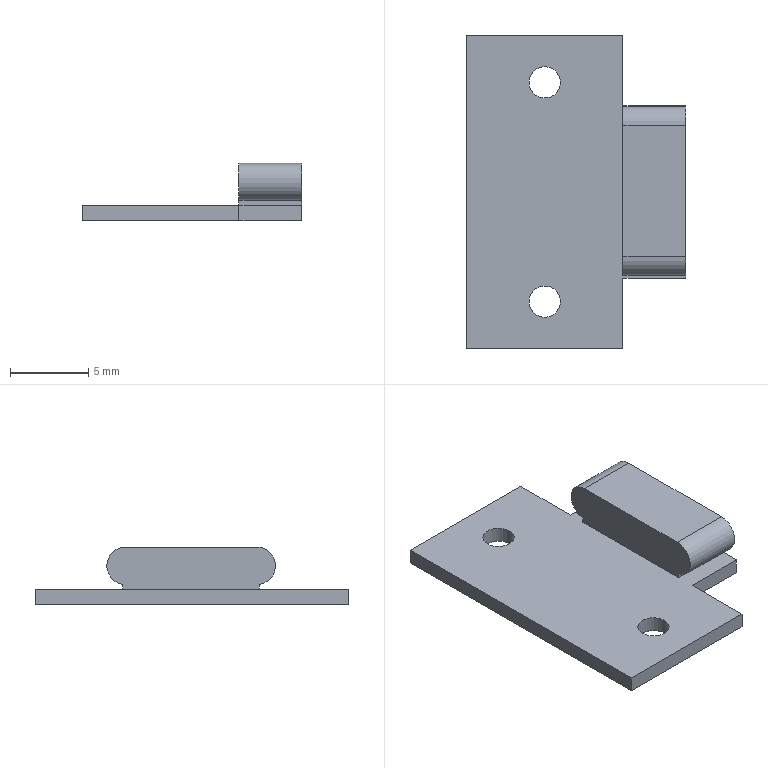Part | SolidWorks | features ICE 4, Extrusion 1 | 1 solid | 25 faces | box 14 x 20 x 3.696 mm | volume 327.493 mm3 | plane 19 | cylinder 6 | commonest cylinder face diameters 2 x4 2.393 x2
STEP:
#1=CARTESIAN_POINT('',(-1.,-7.,1.));
#2=VERTEX_POINT('',#1);
#3=CARTESIAN_POINT('',(1.,-7.,1.));
#4=VERTEX_POINT('',#3);
#5=CARTESIAN_POINT('',(0.,-7.,1.));
#6=DIRECTION('',(0.,0.,1.));
#7=DIRECTION('',(1.,0.,0.));
#8=AXIS2_PLACEMENT_3D('',#5,#6,#7);
#9=CIRCLE('',#8,1.);
#10=EDGE_CURVE('',#2,#4,#9,.T.);
#11=ORIENTED_EDGE('',*,*,#10,.T.);
#12=CARTESIAN_POINT('',(1.,-7.,0.));
#13=VERTEX_POINT('',#12);
#14=CARTESIAN_POINT('',(1.,-7.,1.));
#15=DIRECTION('',(0.,0.,-1.));
#16=VECTOR('',#15,1000.);
#17=LINE('',#14,#16);
#18=EDGE_CURVE('',#4,#13,#17,.T.);
#19=ORIENTED_EDGE('',*,*,#18,.T.);
#20=CARTESIAN_POINT('',(-1.,-7.,0.));
#21=VERTEX_POINT('',#20);
#22=CARTESIAN_POINT('',(0.,-7.,0.));
#23=DIRECTION('',(0.,0.,1.));
#24=DIRECTION('',(1.,0.,0.));
#25=AXIS2_PLACEMENT_3D('',#22,#23,#24);
#26=CIRCLE('',#25,1.);
#27=EDGE_CURVE('',#21,#13,#26,.T.);
#28=ORIENTED_EDGE('',*,*,#27,.F.);
#29=CARTESIAN_POINT('',(-1.,-7.,1.));
#30=DIRECTION('',(0.,0.,-1.));
#31=VECTOR('',#30,1000.);
#32=LINE('',#29,#31);
#33=EDGE_CURVE('',#2,#21,#32,.T.);
#34=ORIENTED_EDGE('',*,*,#33,.F.);
#35=EDGE_LOOP('',(#11,#19,#28,#34));
#36=FACE_OUTER_BOUND('',#35,.T.);
#37=CARTESIAN_POINT('',(0.,-7.,1.));
#38=DIRECTION('',(0.,0.,-1.));
#39=DIRECTION('',(-1.,0.,0.));
#40=AXIS2_PLACEMENT_3D('',#37,#38,#39);
#41=CYLINDRICAL_SURFACE('',#40,1.);
#42=ADVANCED_FACE('',(#36),#41,.F.);
#43=CARTESIAN_POINT('',(-1.,7.,1.));
#44=VERTEX_POINT('',#43);
#45=CARTESIAN_POINT('',(1.,7.,1.));
#46=VERTEX_POINT('',#45);
#47=CARTESIAN_POINT('',(0.,7.,1.));
#48=DIRECTION('',(0.,0.,1.));
#49=DIRECTION('',(1.,0.,0.));
#50=AXIS2_PLACEMENT_3D('',#47,#48,#49);
#51=CIRCLE('',#50,1.);
#52=EDGE_CURVE('',#44,#46,#51,.T.);
#53=ORIENTED_EDGE('',*,*,#52,.T.);
#54=CARTESIAN_POINT('',(1.,7.,0.));
#55=VERTEX_POINT('',#54);
#56=CARTESIAN_POINT('',(1.,7.,1.));
#57=DIRECTION('',(0.,0.,-1.));
#58=VECTOR('',#57,1000.);
#59=LINE('',#56,#58);
#60=EDGE_CURVE('',#46,#55,#59,.T.);
#61=ORIENTED_EDGE('',*,*,#60,.T.);
#62=CARTESIAN_POINT('',(-1.,7.,0.));
#63=VERTEX_POINT('',#62);
#64=CARTESIAN_POINT('',(0.,7.,0.));
#65=DIRECTION('',(0.,0.,1.));
#66=DIRECTION('',(1.,0.,0.));
#67=AXIS2_PLACEMENT_3D('',#64,#65,#66);
#68=CIRCLE('',#67,1.);
#69=EDGE_CURVE('',#63,#55,#68,.T.);
#70=ORIENTED_EDGE('',*,*,#69,.F.);
#71=CARTESIAN_POINT('',(-1.,7.,1.));
#72=DIRECTION('',(0.,0.,-1.));
#73=VECTOR('',#72,1000.);
#74=LINE('',#71,#73);
#75=EDGE_CURVE('',#44,#63,#74,.T.);
#76=ORIENTED_EDGE('',*,*,#75,.F.);
#77=EDGE_LOOP('',(#53,#61,#70,#76));
#78=FACE_OUTER_BOUND('',#77,.T.);
#79=CARTESIAN_POINT('',(0.,7.,1.));
#80=DIRECTION('',(0.,0.,-1.));
#81=DIRECTION('',(-1.,0.,0.));
#82=AXIS2_PLACEMENT_3D('',#79,#80,#81);
#83=CYLINDRICAL_SURFACE('',#82,1.);
#84=ADVANCED_FACE('',(#78),#83,.F.);
#85=CARTESIAN_POINT('',(5.,-4.302,1.));
#86=VERTEX_POINT('',#85);
#87=CARTESIAN_POINT('',(9.,-4.302,1.));
#88=VERTEX_POINT('',#87);
#89=CARTESIAN_POINT('',(5.,-4.302,1.));
#90=DIRECTION('',(1.,0.,0.));
#91=VECTOR('',#90,1000.);
#92=LINE('',#89,#91);
#93=EDGE_CURVE('',#86,#88,#92,.T.);
#94=ORIENTED_EDGE('',*,*,#93,.F.);
#95=CARTESIAN_POINT('',(5.,4.41,1.));
#96=VERTEX_POINT('',#95);
#97=CARTESIAN_POINT('',(5.,-4.302,1.));
#98=DIRECTION('',(0.,1.,0.));
#99=VECTOR('',#98,1000.);
#100=LINE('',#97,#99);
#101=EDGE_CURVE('',#86,#96,#100,.T.);
#102=ORIENTED_EDGE('',*,*,#101,.T.);
#103=CARTESIAN_POINT('',(9.,4.41,1.));
#104=VERTEX_POINT('',#103);
#105=CARTESIAN_POINT('',(5.,4.41,1.));
#106=DIRECTION('',(1.,0.,0.));
#107=VECTOR('',#106,1000.);
#108=LINE('',#105,#107);
#109=EDGE_CURVE('',#96,#104,#108,.T.);
#110=ORIENTED_EDGE('',*,*,#109,.T.);
#111=CARTESIAN_POINT('',(9.,5.5,1.));
#112=VERTEX_POINT('',#111);
#113=CARTESIAN_POINT('',(9.,-5.5,1.));
#114=DIRECTION('',(0.,1.,0.));
#115=VECTOR('',#114,1000.);
#116=LINE('',#113,#115);
#117=EDGE_CURVE('',#104,#112,#116,.T.);
#118=ORIENTED_EDGE('',*,*,#117,.T.);
#119=CARTESIAN_POINT('',(5.,5.5,1.));
#120=VERTEX_POINT('',#119);
#121=CARTESIAN_POINT('',(-1.,5.5,1.));
#122=DIRECTION('',(1.,0.,0.));
#123=VECTOR('',#122,1000.);
#124=LINE('',#121,#123);
#125=EDGE_CURVE('',#120,#112,#124,.T.);
#126=ORIENTED_EDGE('',*,*,#125,.F.);
#127=CARTESIAN_POINT('',(5.,10.,1.));
#128=VERTEX_POINT('',#127);
#129=CARTESIAN_POINT('',(5.,10.,1.));
#130=DIRECTION('',(0.,1.,0.));
#131=VECTOR('',#130,1000.);
#132=LINE('',#129,#131);
#133=EDGE_CURVE('',#120,#128,#132,.T.);
#134=ORIENTED_EDGE('',*,*,#133,.T.);
#135=CARTESIAN_POINT('',(-5.,10.,1.));
#136=VERTEX_POINT('',#135);
#137=CARTESIAN_POINT('',(-5.,10.,1.));
#138=DIRECTION('',(-1.,0.,0.));
#139=VECTOR('',#138,1000.);
#140=LINE('',#137,#139);
#141=EDGE_CURVE('',#128,#136,#140,.T.);
#142=ORIENTED_EDGE('',*,*,#141,.T.);
#143=CARTESIAN_POINT('',(-5.,-10.,1.));
#144=VERTEX_POINT('',#143);
#145=CARTESIAN_POINT('',(-5.,10.,1.));
#146=DIRECTION('',(0.,-1.,0.));
#147=VECTOR('',#146,1000.);
#148=LINE('',#145,#147);
#149=EDGE_CURVE('',#136,#144,#148,.T.);
#150=ORIENTED_EDGE('',*,*,#149,.T.);
#151=CARTESIAN_POINT('',(5.,-10.,1.));
#152=VERTEX_POINT('',#151);
#153=CARTESIAN_POINT('',(-5.,-10.,1.));
#154=DIRECTION('',(1.,0.,0.));
#155=VECTOR('',#154,1000.);
#156=LINE('',#153,#155);
#157=EDGE_CURVE('',#144,#152,#156,.T.);
#158=ORIENTED_EDGE('',*,*,#157,.T.);
#159=CARTESIAN_POINT('',(5.,-5.5,1.));
#160=VERTEX_POINT('',#159);
#161=CARTESIAN_POINT('',(5.,-5.5,1.));
#162=DIRECTION('',(0.,1.,0.));
#163=VECTOR('',#162,1000.);
#164=LINE('',#161,#163);
#165=EDGE_CURVE('',#152,#160,#164,.T.);
#166=ORIENTED_EDGE('',*,*,#165,.T.);
#167=CARTESIAN_POINT('',(9.,-5.5,1.));
#168=VERTEX_POINT('',#167);
#169=CARTESIAN_POINT('',(-1.,-5.5,1.));
#170=DIRECTION('',(1.,0.,0.));
#171=VECTOR('',#170,1000.);
#172=LINE('',#169,#171);
#173=EDGE_CURVE('',#160,#168,#172,.T.);
#174=ORIENTED_EDGE('',*,*,#173,.T.);
#175=CARTESIAN_POINT('',(9.,-5.5,1.));
#176=DIRECTION('',(0.,1.,0.));
#177=VECTOR('',#176,1000.);
#178=LINE('',#175,#177);
#179=EDGE_CURVE('',#168,#88,#178,.T.);
#180=ORIENTED_EDGE('',*,*,#179,.T.);
#181=EDGE_LOOP('',(#94,#102,#110,#118,#126,#134,#142,#150,#158,#166,#174,#180));
#182=FACE_OUTER_BOUND('',#181,.T.);
#183=ORIENTED_EDGE('',*,*,#52,.F.);
#184=CARTESIAN_POINT('',(0.,7.,1.));
#185=DIRECTION('',(0.,0.,1.));
#186=DIRECTION('',(1.,0.,0.));
#187=AXIS2_PLACEMENT_3D('',#184,#185,#186);
#188=CIRCLE('',#187,1.);
#189=EDGE_CURVE('',#46,#44,#188,.T.);
#190=ORIENTED_EDGE('',*,*,#189,.F.);
#191=EDGE_LOOP('',(#183,#190));
#192=FACE_BOUND('',#191,.T.);
#193=ORIENTED_EDGE('',*,*,#10,.F.);
#194=CARTESIAN_POINT('',(0.,-7.,1.));
#195=DIRECTION('',(0.,0.,1.));
#196=DIRECTION('',(1.,0.,0.));
#197=AXIS2_PLACEMENT_3D('',#194,#195,#196);
#198=CIRCLE('',#197,1.);
#199=EDGE_CURVE('',#4,#2,#198,.T.);
#200=ORIENTED_EDGE('',*,*,#199,.F.);
#201=EDGE_LOOP('',(#193,#200));
#202=FACE_BOUND('',#201,.T.);
#203=CARTESIAN_POINT('',(0.,0.,1.));
#204=DIRECTION('',(0.,0.,1.));
#205=DIRECTION('',(1.,0.,0.));
#206=AXIS2_PLACEMENT_3D('',#203,#204,#205);
#207=PLANE('',#206);
#208=ADVANCED_FACE('',(#182,#192,#202),#207,.T.);
#209=CARTESIAN_POINT('',(5.,-10.,0.));
#210=VERTEX_POINT('',#209);
#211=CARTESIAN_POINT('',(5.,-5.5,0.));
#212=VERTEX_POINT('',#211);
#213=CARTESIAN_POINT('',(5.,-5.5,0.));
#214=DIRECTION('',(0.,1.,0.));
#215=VECTOR('',#214,1000.);
#216=LINE('',#213,#215);
#217=EDGE_CURVE('',#210,#212,#216,.T.);
#218=ORIENTED_EDGE('',*,*,#217,.F.);
#219=CARTESIAN_POINT('',(-5.,-10.,0.));
#220=VERTEX_POINT('',#219);
#221=CARTESIAN_POINT('',(-5.,-10.,0.));
#222=DIRECTION('',(1.,0.,0.));
#223=VECTOR('',#222,1000.);
#224=LINE('',#221,#223);
#225=EDGE_CURVE('',#220,#210,#224,.T.);
#226=ORIENTED_EDGE('',*,*,#225,.F.);
#227=CARTESIAN_POINT('',(-5.,10.,0.));
#228=VERTEX_POINT('',#227);
#229=CARTESIAN_POINT('',(-5.,10.,0.));
#230=DIRECTION('',(0.,-1.,0.));
#231=VECTOR('',#230,1000.);
#232=LINE('',#229,#231);
#233=EDGE_CURVE('',#228,#220,#232,.T.);
#234=ORIENTED_EDGE('',*,*,#233,.F.);
#235=CARTESIAN_POINT('',(5.,10.,0.));
#236=VERTEX_POINT('',#235);
#237=CARTESIAN_POINT('',(-5.,10.,0.));
#238=DIRECTION('',(-1.,0.,0.));
#239=VECTOR('',#238,1000.);
#240=LINE('',#237,#239);
#241=EDGE_CURVE('',#236,#228,#240,.T.);
#242=ORIENTED_EDGE('',*,*,#241,.F.);
#243=CARTESIAN_POINT('',(5.,5.5,0.));
#244=VERTEX_POINT('',#243);
#245=CARTESIAN_POINT('',(5.,10.,0.));
#246=DIRECTION('',(0.,1.,0.));
#247=VECTOR('',#246,1000.);
#248=LINE('',#245,#247);
#249=EDGE_CURVE('',#244,#236,#248,.T.);
#250=ORIENTED_EDGE('',*,*,#249,.F.);
#251=CARTESIAN_POINT('',(9.,5.5,0.));
#252=VERTEX_POINT('',#251);
#253=CARTESIAN_POINT('',(5.,5.5,0.));
#254=DIRECTION('',(-1.,0.,0.));
#255=VECTOR('',#254,1000.);
#256=LINE('',#253,#255);
#257=EDGE_CURVE('',#252,#244,#256,.T.);
#258=ORIENTED_EDGE('',*,*,#257,.F.);
#259=CARTESIAN_POINT('',(9.,-5.5,0.));
#260=VERTEX_POINT('',#259);
#261=CARTESIAN_POINT('',(9.,5.5,0.));
#262=DIRECTION('',(0.,1.,0.));
#263=VECTOR('',#262,1000.);
#264=LINE('',#261,#263);
#265=EDGE_CURVE('',#260,#252,#264,.T.);
#266=ORIENTED_EDGE('',*,*,#265,.F.);
#267=CARTESIAN_POINT('',(5.,-5.5,0.));
#268=DIRECTION('',(1.,0.,0.));
#269=VECTOR('',#268,1000.);
#270=LINE('',#267,#269);
#271=EDGE_CURVE('',#212,#260,#270,.T.);
#272=ORIENTED_EDGE('',*,*,#271,.F.);
#273=EDGE_LOOP('',(#218,#226,#234,#242,#250,#258,#266,#272));
#274=FACE_OUTER_BOUND('',#273,.T.);
#275=ORIENTED_EDGE('',*,*,#69,.T.);
#276=CARTESIAN_POINT('',(0.,7.,0.));
#277=DIRECTION('',(0.,0.,1.));
#278=DIRECTION('',(1.,0.,0.));
#279=AXIS2_PLACEMENT_3D('',#276,#277,#278);
#280=CIRCLE('',#279,1.);
#281=EDGE_CURVE('',#55,#63,#280,.T.);
#282=ORIENTED_EDGE('',*,*,#281,.T.);
#283=EDGE_LOOP('',(#275,#282));
#284=FACE_BOUND('',#283,.T.);
#285=ORIENTED_EDGE('',*,*,#27,.T.);
#286=CARTESIAN_POINT('',(0.,-7.,0.));
#287=DIRECTION('',(0.,0.,1.));
#288=DIRECTION('',(1.,0.,0.));
#289=AXIS2_PLACEMENT_3D('',#286,#287,#288);
#290=CIRCLE('',#289,1.);
#291=EDGE_CURVE('',#13,#21,#290,.T.);
#292=ORIENTED_EDGE('',*,*,#291,.T.);
#293=EDGE_LOOP('',(#285,#292));
#294=FACE_BOUND('',#293,.T.);
#295=CARTESIAN_POINT('',(0.,0.,0.));
#296=DIRECTION('',(0.,0.,1.));
#297=DIRECTION('',(1.,0.,0.));
#298=AXIS2_PLACEMENT_3D('',#295,#296,#297);
#299=PLANE('',#298);
#300=ADVANCED_FACE('',(#274,#284,#294),#299,.F.);
#301=ORIENTED_EDGE('',*,*,#217,.T.);
#302=CARTESIAN_POINT('',(5.,-5.5,1.));
#303=DIRECTION('',(0.,0.,-1.));
#304=VECTOR('',#303,1000.);
#305=LINE('',#302,#304);
#306=EDGE_CURVE('',#160,#212,#305,.T.);
#307=ORIENTED_EDGE('',*,*,#306,.F.);
#308=ORIENTED_EDGE('',*,*,#165,.F.);
#309=CARTESIAN_POINT('',(5.,-10.,1.));
#310=DIRECTION('',(0.,0.,-1.));
#311=VECTOR('',#310,1000.);
#312=LINE('',#309,#311);
#313=EDGE_CURVE('',#152,#210,#312,.T.);
#314=ORIENTED_EDGE('',*,*,#313,.T.);
#315=EDGE_LOOP('',(#301,#307,#308,#314));
#316=FACE_OUTER_BOUND('',#315,.T.);
#317=CARTESIAN_POINT('',(5.,-5.5,1.));
#318=DIRECTION('',(-1.,0.,0.));
#319=DIRECTION('',(0.,-1.,0.));
#320=AXIS2_PLACEMENT_3D('',#317,#318,#319);
#321=PLANE('',#320);
#322=ADVANCED_FACE('',(#316),#321,.F.);
#323=CARTESIAN_POINT('',(9.,-5.5,1.));
#324=DIRECTION('',(0.,0.,-1.));
#325=VECTOR('',#324,1000.);
#326=LINE('',#323,#325);
#327=EDGE_CURVE('',#168,#260,#326,.T.);
#328=ORIENTED_EDGE('',*,*,#327,.F.);
#329=ORIENTED_EDGE('',*,*,#173,.F.);
#330=ORIENTED_EDGE('',*,*,#306,.T.);
#331=ORIENTED_EDGE('',*,*,#271,.T.);
#332=EDGE_LOOP('',(#328,#329,#330,#331));
#333=FACE_OUTER_BOUND('',#332,.T.);
#334=CARTESIAN_POINT('',(5.,-5.5,1.));
#335=DIRECTION('',(0.,1.,0.));
#336=DIRECTION('',(-1.,0.,0.));
#337=AXIS2_PLACEMENT_3D('',#334,#335,#336);
#338=PLANE('',#337);
#339=ADVANCED_FACE('',(#333),#338,.F.);
#340=CARTESIAN_POINT('',(9.,-4.14,3.696));
#341=VERTEX_POINT('',#340);
#342=CARTESIAN_POINT('',(9.,-4.302,1.315));
#343=VERTEX_POINT('',#342);
#344=CARTESIAN_POINT('',(9.,-4.14,2.5));
#345=DIRECTION('',(1.,0.,0.));
#346=DIRECTION('',(0.,0.,-1.));
#347=AXIS2_PLACEMENT_3D('',#344,#345,#346);
#348=CIRCLE('',#347,1.196);
#349=EDGE_CURVE('',#341,#343,#348,.T.);
#350=ORIENTED_EDGE('',*,*,#349,.T.);
#351=CARTESIAN_POINT('',(9.,-4.302,1.607));
#352=DIRECTION('',(0.,0.,-1.));
#353=VECTOR('',#352,1000.);
#354=LINE('',#351,#353);
#355=EDGE_CURVE('',#343,#88,#354,.T.);
#356=ORIENTED_EDGE('',*,*,#355,.T.);
#357=ORIENTED_EDGE('',*,*,#179,.F.);
#358=ORIENTED_EDGE('',*,*,#327,.T.);
#359=ORIENTED_EDGE('',*,*,#265,.T.);
#360=CARTESIAN_POINT('',(9.,5.5,1.));
#361=DIRECTION('',(0.,0.,-1.));
#362=VECTOR('',#361,1000.);
#363=LINE('',#360,#362);
#364=EDGE_CURVE('',#112,#252,#363,.T.);
#365=ORIENTED_EDGE('',*,*,#364,.F.);
#366=ORIENTED_EDGE('',*,*,#117,.F.);
#367=CARTESIAN_POINT('',(9.,4.41,1.315));
#368=VERTEX_POINT('',#367);
#369=CARTESIAN_POINT('',(9.,4.41,1.607));
#370=DIRECTION('',(0.,0.,1.));
#371=VECTOR('',#370,1000.);
#372=LINE('',#369,#371);
#373=EDGE_CURVE('',#104,#368,#372,.T.);
#374=ORIENTED_EDGE('',*,*,#373,.T.);
#375=CARTESIAN_POINT('',(9.,4.248,3.696));
#376=VERTEX_POINT('',#375);
#377=CARTESIAN_POINT('',(9.,4.248,2.5));
#378=DIRECTION('',(1.,0.,0.));
#379=DIRECTION('',(0.,0.,-1.));
#380=AXIS2_PLACEMENT_3D('',#377,#378,#379);
#381=CIRCLE('',#380,1.196);
#382=EDGE_CURVE('',#368,#376,#381,.T.);
#383=ORIENTED_EDGE('',*,*,#382,.T.);
#384=CARTESIAN_POINT('',(9.,4.248,3.696));
#385=DIRECTION('',(0.,-1.,0.));
#386=VECTOR('',#385,1000.);
#387=LINE('',#384,#386);
#388=EDGE_CURVE('',#376,#341,#387,.T.);
#389=ORIENTED_EDGE('',*,*,#388,.T.);
#390=EDGE_LOOP('',(#350,#356,#357,#358,#359,#365,#366,#374,#383,#389));
#391=FACE_OUTER_BOUND('',#390,.T.);
#392=CARTESIAN_POINT('',(9.,4.573,2.105));
#393=VERTEX_POINT('',#392);
#394=CARTESIAN_POINT('',(9.,4.573,2.809));
#395=VERTEX_POINT('',#394);
#396=CARTESIAN_POINT('',(9.,4.573,2.809));
#397=DIRECTION('',(0.,0.,1.));
#398=VECTOR('',#397,1000.);
#399=LINE('',#396,#398);
#400=EDGE_CURVE('',#393,#395,#399,.T.);
#401=ORIENTED_EDGE('',*,*,#400,.F.);
#402=CARTESIAN_POINT('',(9.,-4.464,2.105));
#403=VERTEX_POINT('',#402);
#404=CARTESIAN_POINT('',(9.,4.573,2.105));
#405=DIRECTION('',(0.,1.,0.));
#406=VECTOR('',#405,1000.);
#407=LINE('',#404,#406);
#408=EDGE_CURVE('',#403,#393,#407,.T.);
#409=ORIENTED_EDGE('',*,*,#408,.F.);
#410=CARTESIAN_POINT('',(9.,-4.464,2.809));
#411=VERTEX_POINT('',#410);
#412=CARTESIAN_POINT('',(9.,-4.464,2.809));
#413=DIRECTION('',(0.,0.,-1.));
#414=VECTOR('',#413,1000.);
#415=LINE('',#412,#414);
#416=EDGE_CURVE('',#411,#403,#415,.T.);
#417=ORIENTED_EDGE('',*,*,#416,.F.);
#418=CARTESIAN_POINT('',(9.,4.573,2.809));
#419=DIRECTION('',(0.,-1.,0.));
#420=VECTOR('',#419,1000.);
#421=LINE('',#418,#420);
#422=EDGE_CURVE('',#395,#411,#421,.T.);
#423=ORIENTED_EDGE('',*,*,#422,.F.);
#424=EDGE_LOOP('',(#401,#409,#417,#423));
#425=FACE_BOUND('',#424,.T.);
#426=CARTESIAN_POINT('',(9.,5.5,1.));
#427=DIRECTION('',(-1.,0.,0.));
#428=DIRECTION('',(0.,0.,1.));
#429=AXIS2_PLACEMENT_3D('',#426,#427,#428);
#430=PLANE('',#429);
#431=ADVANCED_FACE('',(#391,#425),#430,.F.);
#432=CARTESIAN_POINT('',(5.,5.5,1.));
#433=DIRECTION('',(0.,0.,-1.));
#434=VECTOR('',#433,1000.);
#435=LINE('',#432,#434);
#436=EDGE_CURVE('',#120,#244,#435,.T.);
#437=ORIENTED_EDGE('',*,*,#436,.F.);
#438=ORIENTED_EDGE('',*,*,#125,.T.);
#439=ORIENTED_EDGE('',*,*,#364,.T.);
#440=ORIENTED_EDGE('',*,*,#257,.T.);
#441=EDGE_LOOP('',(#437,#438,#439,#440));
#442=FACE_OUTER_BOUND('',#441,.T.);
#443=CARTESIAN_POINT('',(5.,5.5,1.));
#444=DIRECTION('',(0.,-1.,0.));
#445=DIRECTION('',(0.,0.,-1.));
#446=AXIS2_PLACEMENT_3D('',#443,#444,#445);
#447=PLANE('',#446);
#448=ADVANCED_FACE('',(#442),#447,.F.);
#449=ORIENTED_EDGE('',*,*,#249,.T.);
#450=CARTESIAN_POINT('',(5.,10.,1.));
#451=DIRECTION('',(0.,0.,-1.));
#452=VECTOR('',#451,1000.);
#453=LINE('',#450,#452);
#454=EDGE_CURVE('',#128,#236,#453,.T.);
#455=ORIENTED_EDGE('',*,*,#454,.F.);
#456=ORIENTED_EDGE('',*,*,#133,.F.);
#457=ORIENTED_EDGE('',*,*,#436,.T.);
#458=EDGE_LOOP('',(#449,#455,#456,#457));
#459=FACE_OUTER_BOUND('',#458,.T.);
#460=CARTESIAN_POINT('',(5.,10.,1.));
#461=DIRECTION('',(-1.,0.,0.));
#462=DIRECTION('',(0.,-1.,0.));
#463=AXIS2_PLACEMENT_3D('',#460,#461,#462);
#464=PLANE('',#463);
#465=ADVANCED_FACE('',(#459),#464,.F.);
#466=ORIENTED_EDGE('',*,*,#241,.T.);
#467=CARTESIAN_POINT('',(-5.,10.,1.));
#468=DIRECTION('',(0.,0.,-1.));
#469=VECTOR('',#468,1000.);
#470=LINE('',#467,#469);
#471=EDGE_CURVE('',#136,#228,#470,.T.);
#472=ORIENTED_EDGE('',*,*,#471,.F.);
#473=ORIENTED_EDGE('',*,*,#141,.F.);
#474=ORIENTED_EDGE('',*,*,#454,.T.);
#475=EDGE_LOOP('',(#466,#472,#473,#474));
#476=FACE_OUTER_BOUND('',#475,.T.);
#477=CARTESIAN_POINT('',(-5.,10.,1.));
#478=DIRECTION('',(0.,-1.,0.));
#479=DIRECTION('',(0.,0.,-1.));
#480=AXIS2_PLACEMENT_3D('',#477,#478,#479);
#481=PLANE('',#480);
#482=ADVANCED_FACE('',(#476),#481,.F.);
#483=ORIENTED_EDGE('',*,*,#233,.T.);
#484=CARTESIAN_POINT('',(-5.,-10.,1.));
#485=DIRECTION('',(0.,0.,-1.));
#486=VECTOR('',#485,1000.);
#487=LINE('',#484,#486);
#488=EDGE_CURVE('',#144,#220,#487,.T.);
#489=ORIENTED_EDGE('',*,*,#488,.F.);
#490=ORIENTED_EDGE('',*,*,#149,.F.);
#491=ORIENTED_EDGE('',*,*,#471,.T.);
#492=EDGE_LOOP('',(#483,#489,#490,#491));
#493=FACE_OUTER_BOUND('',#492,.T.);
#494=CARTESIAN_POINT('',(-5.,10.,1.));
#495=DIRECTION('',(1.,0.,0.));
#496=DIRECTION('',(0.,1.,0.));
#497=AXIS2_PLACEMENT_3D('',#494,#495,#496);
#498=PLANE('',#497);
#499=ADVANCED_FACE('',(#493),#498,.F.);
#500=ORIENTED_EDGE('',*,*,#225,.T.);
#501=ORIENTED_EDGE('',*,*,#313,.F.);
#502=ORIENTED_EDGE('',*,*,#157,.F.);
#503=ORIENTED_EDGE('',*,*,#488,.T.);
#504=EDGE_LOOP('',(#500,#501,#502,#503));
#505=FACE_OUTER_BOUND('',#504,.T.);
#506=CARTESIAN_POINT('',(-5.,-10.,1.));
#507=DIRECTION('',(0.,1.,0.));
#508=DIRECTION('',(0.,0.,1.));
#509=AXIS2_PLACEMENT_3D('',#506,#507,#508);
#510=PLANE('',#509);
#511=ADVANCED_FACE('',(#505),#510,.F.);
#512=ORIENTED_EDGE('',*,*,#60,.F.);
#513=ORIENTED_EDGE('',*,*,#189,.T.);
#514=ORIENTED_EDGE('',*,*,#75,.T.);
#515=ORIENTED_EDGE('',*,*,#281,.F.);
#516=EDGE_LOOP('',(#512,#513,#514,#515));
#517=FACE_OUTER_BOUND('',#516,.T.);
#518=CARTESIAN_POINT('',(0.,7.,1.));
#519=DIRECTION('',(0.,0.,-1.));
#520=DIRECTION('',(-1.,0.,0.));
#521=AXIS2_PLACEMENT_3D('',#518,#519,#520);
#522=CYLINDRICAL_SURFACE('',#521,1.);
#523=ADVANCED_FACE('',(#517),#522,.F.);
#524=ORIENTED_EDGE('',*,*,#18,.F.);
#525=ORIENTED_EDGE('',*,*,#199,.T.);
#526=ORIENTED_EDGE('',*,*,#33,.T.);
#527=ORIENTED_EDGE('',*,*,#291,.F.);
#528=EDGE_LOOP('',(#524,#525,#526,#527));
#529=FACE_OUTER_BOUND('',#528,.T.);
#530=CARTESIAN_POINT('',(0.,-7.,1.));
#531=DIRECTION('',(0.,0.,-1.));
#532=DIRECTION('',(-1.,0.,0.));
#533=AXIS2_PLACEMENT_3D('',#530,#531,#532);
#534=CYLINDRICAL_SURFACE('',#533,1.);
#535=ADVANCED_FACE('',(#529),#534,.F.);
#536=CARTESIAN_POINT('',(5.,-4.302,1.315));
#537=VERTEX_POINT('',#536);
#538=CARTESIAN_POINT('',(-1.,-4.302,1.315));
#539=DIRECTION('',(1.,0.,0.));
#540=VECTOR('',#539,1000.);
#541=LINE('',#538,#540);
#542=EDGE_CURVE('',#537,#343,#541,.T.);
#543=ORIENTED_EDGE('',*,*,#542,.F.);
#544=CARTESIAN_POINT('',(5.,-4.302,1.607));
#545=DIRECTION('',(0.,0.,-1.));
#546=VECTOR('',#545,1000.);
#547=LINE('',#544,#546);
#548=EDGE_CURVE('',#537,#86,#547,.T.);
#549=ORIENTED_EDGE('',*,*,#548,.T.);
#550=ORIENTED_EDGE('',*,*,#93,.T.);
#551=ORIENTED_EDGE('',*,*,#355,.F.);
#552=EDGE_LOOP('',(#543,#549,#550,#551));
#553=FACE_OUTER_BOUND('',#552,.T.);
#554=CARTESIAN_POINT('',(5.,-4.302,1.607));
#555=DIRECTION('',(0.,-1.,0.));
#556=DIRECTION('',(0.,0.,-1.));
#557=AXIS2_PLACEMENT_3D('',#554,#555,#556);
#558=PLANE('',#557);
#559=ADVANCED_FACE('',(#553),#558,.T.);
#560=CARTESIAN_POINT('',(5.,4.41,1.315));
#561=VERTEX_POINT('',#560);
#562=CARTESIAN_POINT('',(-1.,4.41,1.315));
#563=DIRECTION('',(-1.,0.,0.));
#564=VECTOR('',#563,1000.);
#565=LINE('',#562,#564);
#566=EDGE_CURVE('',#368,#561,#565,.T.);
#567=ORIENTED_EDGE('',*,*,#566,.F.);
#568=ORIENTED_EDGE('',*,*,#373,.F.);
#569=ORIENTED_EDGE('',*,*,#109,.F.);
#570=CARTESIAN_POINT('',(5.,4.41,1.607));
#571=DIRECTION('',(0.,0.,1.));
#572=VECTOR('',#571,1000.);
#573=LINE('',#570,#572);
#574=EDGE_CURVE('',#96,#561,#573,.T.);
#575=ORIENTED_EDGE('',*,*,#574,.T.);
#576=EDGE_LOOP('',(#567,#568,#569,#575));
#577=FACE_OUTER_BOUND('',#576,.T.);
#578=CARTESIAN_POINT('',(5.,4.41,1.607));
#579=DIRECTION('',(0.,1.,0.));
#580=DIRECTION('',(0.,0.,1.));
#581=AXIS2_PLACEMENT_3D('',#578,#579,#580);
#582=PLANE('',#581);
#583=ADVANCED_FACE('',(#577),#582,.T.);
#584=ORIENTED_EDGE('',*,*,#548,.F.);
#585=CARTESIAN_POINT('',(5.,-4.14,3.696));
#586=VERTEX_POINT('',#585);
#587=CARTESIAN_POINT('',(5.,-4.14,2.5));
#588=DIRECTION('',(1.,0.,0.));
#589=DIRECTION('',(0.,1.,0.));
#590=AXIS2_PLACEMENT_3D('',#587,#588,#589);
#591=CIRCLE('',#590,1.196);
#592=EDGE_CURVE('',#586,#537,#591,.T.);
#593=ORIENTED_EDGE('',*,*,#592,.F.);
#594=CARTESIAN_POINT('',(5.,4.248,3.696));
#595=VERTEX_POINT('',#594);
#596=CARTESIAN_POINT('',(5.,5.5,3.696));
#597=DIRECTION('',(0.,-1.,0.));
#598=VECTOR('',#597,1000.);
#599=LINE('',#596,#598);
#600=EDGE_CURVE('',#595,#586,#599,.T.);
#601=ORIENTED_EDGE('',*,*,#600,.F.);
#602=CARTESIAN_POINT('',(5.,4.248,2.5));
#603=DIRECTION('',(1.,0.,0.));
#604=DIRECTION('',(0.,1.,0.));
#605=AXIS2_PLACEMENT_3D('',#602,#603,#604);
#606=CIRCLE('',#605,1.196);
#607=EDGE_CURVE('',#561,#595,#606,.T.);
#608=ORIENTED_EDGE('',*,*,#607,.F.);
#609=ORIENTED_EDGE('',*,*,#574,.F.);
#610=ORIENTED_EDGE('',*,*,#101,.F.);
#611=EDGE_LOOP('',(#584,#593,#601,#608,#609,#610));
#612=FACE_OUTER_BOUND('',#611,.T.);
#613=CARTESIAN_POINT('',(5.,0.,0.));
#614=DIRECTION('',(-1.,0.,0.));
#615=DIRECTION('',(0.,0.,1.));
#616=AXIS2_PLACEMENT_3D('',#613,#614,#615);
#617=PLANE('',#616);
#618=ADVANCED_FACE('',(#612),#617,.T.);
#619=ORIENTED_EDGE('',*,*,#600,.T.);
#620=CARTESIAN_POINT('',(-1.,-4.14,3.696));
#621=DIRECTION('',(1.,0.,0.));
#622=VECTOR('',#621,1000.);
#623=LINE('',#620,#622);
#624=EDGE_CURVE('',#586,#341,#623,.T.);
#625=ORIENTED_EDGE('',*,*,#624,.T.);
#626=ORIENTED_EDGE('',*,*,#388,.F.);
#627=CARTESIAN_POINT('',(-1.,4.248,3.696));
#628=DIRECTION('',(1.,0.,0.));
#629=VECTOR('',#628,1000.);
#630=LINE('',#627,#629);
#631=EDGE_CURVE('',#595,#376,#630,.T.);
#632=ORIENTED_EDGE('',*,*,#631,.F.);
#633=EDGE_LOOP('',(#619,#625,#626,#632));
#634=FACE_OUTER_BOUND('',#633,.T.);
#635=CARTESIAN_POINT('',(-1.,4.248,3.696));
#636=DIRECTION('',(0.,0.,1.));
#637=DIRECTION('',(0.,-1.,0.));
#638=AXIS2_PLACEMENT_3D('',#635,#636,#637);
#639=PLANE('',#638);
#640=ADVANCED_FACE('',(#634),#639,.T.);
#641=ORIENTED_EDGE('',*,*,#592,.T.);
#642=ORIENTED_EDGE('',*,*,#542,.T.);
#643=ORIENTED_EDGE('',*,*,#349,.F.);
#644=ORIENTED_EDGE('',*,*,#624,.F.);
#645=EDGE_LOOP('',(#641,#642,#643,#644));
#646=FACE_OUTER_BOUND('',#645,.T.);
#647=CARTESIAN_POINT('',(-1.,-4.14,2.5));
#648=DIRECTION('',(1.,0.,0.));
#649=DIRECTION('',(0.,0.,-1.));
#650=AXIS2_PLACEMENT_3D('',#647,#648,#649);
#651=CYLINDRICAL_SURFACE('',#650,1.196);
#652=ADVANCED_FACE('',(#646),#651,.T.);
#653=ORIENTED_EDGE('',*,*,#382,.F.);
#654=ORIENTED_EDGE('',*,*,#566,.T.);
#655=ORIENTED_EDGE('',*,*,#607,.T.);
#656=ORIENTED_EDGE('',*,*,#631,.T.);
#657=EDGE_LOOP('',(#653,#654,#655,#656));
#658=FACE_OUTER_BOUND('',#657,.T.);
#659=CARTESIAN_POINT('',(-1.,4.248,2.5));
#660=DIRECTION('',(1.,0.,0.));
#661=DIRECTION('',(0.,0.,-1.));
#662=AXIS2_PLACEMENT_3D('',#659,#660,#661);
#663=CYLINDRICAL_SURFACE('',#662,1.196);
#664=ADVANCED_FACE('',(#658),#663,.T.);
#665=ORIENTED_EDGE('',*,*,#408,.T.);
#666=CARTESIAN_POINT('',(6.,4.573,2.105));
#667=VERTEX_POINT('',#666);
#668=CARTESIAN_POINT('',(6.,4.573,2.105));
#669=DIRECTION('',(1.,0.,0.));
#670=VECTOR('',#669,1000.);
#671=LINE('',#668,#670);
#672=EDGE_CURVE('',#667,#393,#671,.T.);
#673=ORIENTED_EDGE('',*,*,#672,.F.);
#674=CARTESIAN_POINT('',(6.,-4.464,2.105));
#675=VERTEX_POINT('',#674);
#676=CARTESIAN_POINT('',(6.,4.573,2.105));
#677=DIRECTION('',(0.,1.,0.));
#678=VECTOR('',#677,1000.);
#679=LINE('',#676,#678);
#680=EDGE_CURVE('',#675,#667,#679,.T.);
#681=ORIENTED_EDGE('',*,*,#680,.F.);
#682=CARTESIAN_POINT('',(6.,-4.464,2.105));
#683=DIRECTION('',(1.,0.,0.));
#684=VECTOR('',#683,1000.);
#685=LINE('',#682,#684);
#686=EDGE_CURVE('',#675,#403,#685,.T.);
#687=ORIENTED_EDGE('',*,*,#686,.T.);
#688=EDGE_LOOP('',(#665,#673,#681,#687));
#689=FACE_OUTER_BOUND('',#688,.T.);
#690=CARTESIAN_POINT('',(6.,4.573,2.105));
#691=DIRECTION('',(0.,0.,-1.));
#692=DIRECTION('',(-1.,0.,0.));
#693=AXIS2_PLACEMENT_3D('',#690,#691,#692);
#694=PLANE('',#693);
#695=ADVANCED_FACE('',(#689),#694,.F.);
#696=ORIENTED_EDGE('',*,*,#416,.T.);
#697=ORIENTED_EDGE('',*,*,#686,.F.);
#698=CARTESIAN_POINT('',(6.,-4.464,2.809));
#699=VERTEX_POINT('',#698);
#700=CARTESIAN_POINT('',(6.,-4.464,2.809));
#701=DIRECTION('',(0.,0.,-1.));
#702=VECTOR('',#701,1000.);
#703=LINE('',#700,#702);
#704=EDGE_CURVE('',#699,#675,#703,.T.);
#705=ORIENTED_EDGE('',*,*,#704,.F.);
#706=CARTESIAN_POINT('',(6.,-4.464,2.809));
#707=DIRECTION('',(1.,0.,0.));
#708=VECTOR('',#707,1000.);
#709=LINE('',#706,#708);
#710=EDGE_CURVE('',#699,#411,#709,.T.);
#711=ORIENTED_EDGE('',*,*,#710,.T.);
#712=EDGE_LOOP('',(#696,#697,#705,#711));
#713=FACE_OUTER_BOUND('',#712,.T.);
#714=CARTESIAN_POINT('',(6.,-4.464,2.809));
#715=DIRECTION('',(0.,-1.,0.));
#716=DIRECTION('',(0.,0.,-1.));
#717=AXIS2_PLACEMENT_3D('',#714,#715,#716);
#718=PLANE('',#717);
#719=ADVANCED_FACE('',(#713),#718,.F.);
#720=ORIENTED_EDGE('',*,*,#422,.T.);
#721=ORIENTED_EDGE('',*,*,#710,.F.);
#722=CARTESIAN_POINT('',(6.,4.573,2.809));
#723=VERTEX_POINT('',#722);
#724=CARTESIAN_POINT('',(6.,4.573,2.809));
#725=DIRECTION('',(0.,-1.,0.));
#726=VECTOR('',#725,1000.);
#727=LINE('',#724,#726);
#728=EDGE_CURVE('',#723,#699,#727,.T.);
#729=ORIENTED_EDGE('',*,*,#728,.F.);
#730=CARTESIAN_POINT('',(6.,4.573,2.809));
#731=DIRECTION('',(1.,0.,0.));
#732=VECTOR('',#731,1000.);
#733=LINE('',#730,#732);
#734=EDGE_CURVE('',#723,#395,#733,.T.);
#735=ORIENTED_EDGE('',*,*,#734,.T.);
#736=EDGE_LOOP('',(#720,#721,#729,#735));
#737=FACE_OUTER_BOUND('',#736,.T.);
#738=CARTESIAN_POINT('',(6.,4.573,2.809));
#739=DIRECTION('',(0.,0.,1.));
#740=DIRECTION('',(1.,0.,0.));
#741=AXIS2_PLACEMENT_3D('',#738,#739,#740);
#742=PLANE('',#741);
#743=ADVANCED_FACE('',(#737),#742,.F.);
#744=ORIENTED_EDGE('',*,*,#400,.T.);
#745=ORIENTED_EDGE('',*,*,#734,.F.);
#746=CARTESIAN_POINT('',(6.,4.573,2.809));
#747=DIRECTION('',(0.,0.,1.));
#748=VECTOR('',#747,1000.);
#749=LINE('',#746,#748);
#750=EDGE_CURVE('',#667,#723,#749,.T.);
#751=ORIENTED_EDGE('',*,*,#750,.F.);
#752=ORIENTED_EDGE('',*,*,#672,.T.);
#753=EDGE_LOOP('',(#744,#745,#751,#752));
#754=FACE_OUTER_BOUND('',#753,.T.);
#755=CARTESIAN_POINT('',(6.,4.573,2.809));
#756=DIRECTION('',(0.,1.,0.));
#757=DIRECTION('',(0.,0.,1.));
#758=AXIS2_PLACEMENT_3D('',#755,#756,#757);
#759=PLANE('',#758);
#760=ADVANCED_FACE('',(#754),#759,.F.);
#761=ORIENTED_EDGE('',*,*,#680,.T.);
#762=ORIENTED_EDGE('',*,*,#750,.T.);
#763=ORIENTED_EDGE('',*,*,#728,.T.);
#764=ORIENTED_EDGE('',*,*,#704,.T.);
#765=EDGE_LOOP('',(#761,#762,#763,#764));
#766=FACE_OUTER_BOUND('',#765,.T.);
#767=CARTESIAN_POINT('',(6.,0.,0.));
#768=DIRECTION('',(1.,0.,0.));
#769=DIRECTION('',(0.,0.,-1.));
#770=AXIS2_PLACEMENT_3D('',#767,#768,#769);
#771=PLANE('',#770);
#772=ADVANCED_FACE('',(#766),#771,.T.);
#773=CLOSED_SHELL('',(#42,#84,#208,#300,#322,#339,#431,#448,#465,#482,#499,#511,#523,#535,#559,#583,#618,#640,#652,#664,#695,#719,#743,#760,#772));
#774=MANIFOLD_SOLID_BREP('',#773);
#775=CARTESIAN_POINT('',(0.,0.,0.));
#776=DIRECTION('',(0.,0.,1.));
#777=DIRECTION('',(1.,0.,0.));
#778=AXIS2_PLACEMENT_3D('',#775,#776,#777);
#779=(LENGTH_UNIT()NAMED_UNIT(*)SI_UNIT(.MILLI.,.METRE.));
#780=UNCERTAINTY_MEASURE_WITH_UNIT(LENGTH_MEASURE(0.00001),#779,'','');
#781=(NAMED_UNIT(*)PLANE_ANGLE_UNIT()SI_UNIT($,.RADIAN.));
#782=(NAMED_UNIT(*)SI_UNIT($,.STERADIAN.)SOLID_ANGLE_UNIT());
#783=(GEOMETRIC_REPRESENTATION_CONTEXT(3)GLOBAL_UNCERTAINTY_ASSIGNED_CONTEXT((#780))GLOBAL_UNIT_ASSIGNED_CONTEXT((#779,#781,#782))REPRESENTATION_CONTEXT('',''));
#784=ADVANCED_BREP_SHAPE_REPRESENTATION('',(#774,#778),#783);